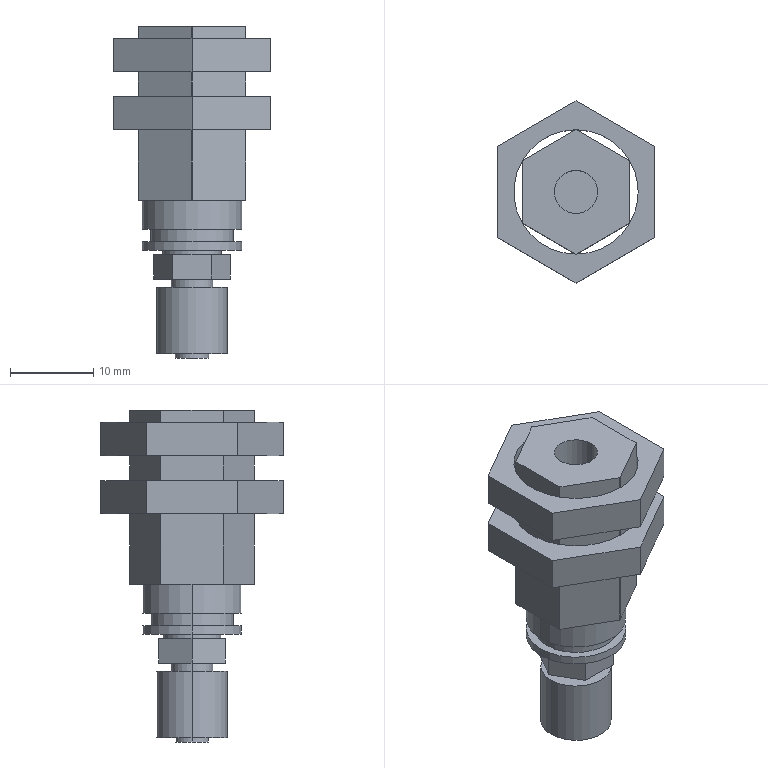Part | STEP file | body_A_CJPB10_10_H4_0_ | 1 solid | 93 faces | box 19 x 21.939 x 40 mm | volume 5154 mm3 | plane 59 | cylinder 32 | cone 2 | commonest cylinder face diameters 14.98 x14 12 x4 4 x2 4.13 x2 5 x2 5.2 x2